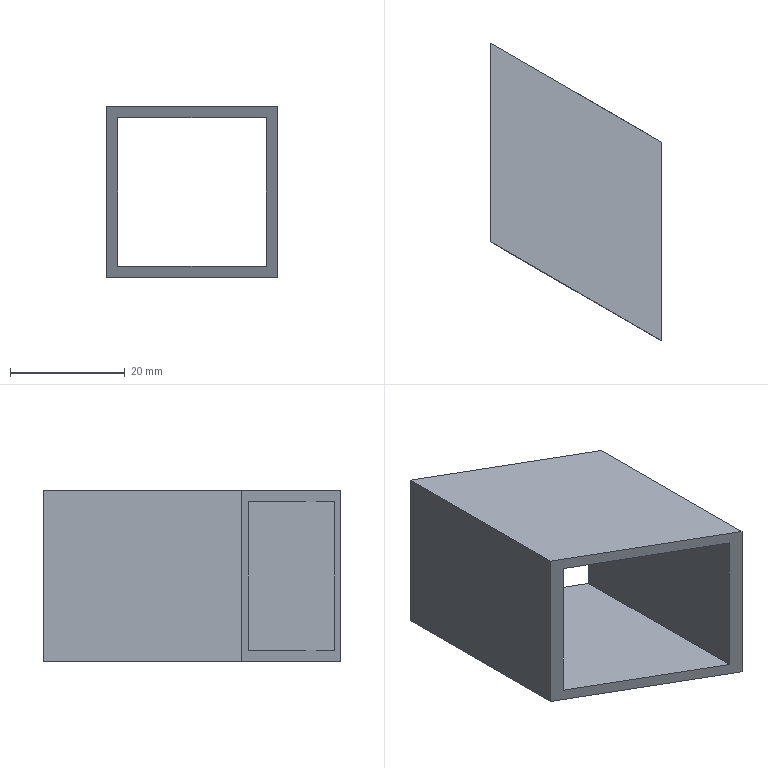Part | NX | features solid 2 | 1 solid | 10 faces | box 30 x 51.962 x 30 mm | volume 7760 mm3 | plane 10
STEP:
#1=CARTESIAN_POINT('',(242.,-18.46,-73.));
#2=VERTEX_POINT('',#1);
#3=CARTESIAN_POINT('',(242.,-18.46,-47.));
#4=VERTEX_POINT('',#3);
#5=CARTESIAN_POINT('',(242.,-18.46,-75.));
#6=DIRECTION('',(0.,0.,1.));
#7=VECTOR('',#6,1000.);
#8=LINE('',#5,#7);
#9=EDGE_CURVE('',#2,#4,#8,.T.);
#10=ORIENTED_EDGE('',*,*,#9,.F.);
#11=CARTESIAN_POINT('',(268.,-33.471,-73.));
#12=VERTEX_POINT('',#11);
#13=CARTESIAN_POINT('',(237.686,-15.97,-73.));
#14=DIRECTION('',(0.866,-0.5,0.));
#15=VECTOR('',#14,1000.);
#16=LINE('',#13,#15);
#17=EDGE_CURVE('',#12,#2,#16,.F.);
#18=ORIENTED_EDGE('',*,*,#17,.F.);
#19=CARTESIAN_POINT('',(268.,-33.471,-47.));
#20=VERTEX_POINT('',#19);
#21=CARTESIAN_POINT('',(268.,-33.471,-75.));
#22=DIRECTION('',(0.,0.,1.));
#23=VECTOR('',#22,1000.);
#24=LINE('',#21,#23);
#25=EDGE_CURVE('',#12,#20,#24,.T.);
#26=ORIENTED_EDGE('',*,*,#25,.T.);
#27=CARTESIAN_POINT('',(237.686,-15.97,-47.));
#28=DIRECTION('',(0.866,-0.5,0.));
#29=VECTOR('',#28,1000.);
#30=LINE('',#27,#29);
#31=EDGE_CURVE('',#4,#20,#30,.T.);
#32=ORIENTED_EDGE('',*,*,#31,.F.);
#33=EDGE_LOOP('',(#10,#18,#26,#32));
#34=FACE_BOUND('',#33,.T.);
#35=CARTESIAN_POINT('',(270.,-34.626,-75.));
#36=VERTEX_POINT('',#35);
#37=CARTESIAN_POINT('',(240.,-17.306,-75.));
#38=VERTEX_POINT('',#37);
#39=CARTESIAN_POINT('',(237.686,-15.97,-75.));
#40=DIRECTION('',(0.866,-0.5,0.));
#41=VECTOR('',#40,1000.);
#42=LINE('',#39,#41);
#43=EDGE_CURVE('',#36,#38,#42,.F.);
#44=ORIENTED_EDGE('',*,*,#43,.T.);
#45=CARTESIAN_POINT('',(240.,-17.306,-45.));
#46=VERTEX_POINT('',#45);
#47=CARTESIAN_POINT('',(240.,-17.306,-75.));
#48=DIRECTION('',(0.,0.,1.));
#49=VECTOR('',#48,1000.);
#50=LINE('',#47,#49);
#51=EDGE_CURVE('',#38,#46,#50,.T.);
#52=ORIENTED_EDGE('',*,*,#51,.T.);
#53=CARTESIAN_POINT('',(270.,-34.626,-45.));
#54=VERTEX_POINT('',#53);
#55=CARTESIAN_POINT('',(237.686,-15.97,-45.));
#56=DIRECTION('',(0.866,-0.5,0.));
#57=VECTOR('',#56,1000.);
#58=LINE('',#55,#57);
#59=EDGE_CURVE('',#46,#54,#58,.T.);
#60=ORIENTED_EDGE('',*,*,#59,.T.);
#61=CARTESIAN_POINT('',(270.,-34.626,-75.));
#62=DIRECTION('',(0.,0.,1.));
#63=VECTOR('',#62,1000.);
#64=LINE('',#61,#63);
#65=EDGE_CURVE('',#36,#54,#64,.T.);
#66=ORIENTED_EDGE('',*,*,#65,.F.);
#67=EDGE_LOOP('',(#44,#52,#60,#66));
#68=FACE_BOUND('',#67,.T.);
#69=CARTESIAN_POINT('',(476.795,-154.019,-105.));
#70=DIRECTION('',(0.5,0.866,0.));
#71=DIRECTION('',(0.,0.,-1.));
#72=AXIS2_PLACEMENT_3D('',#69,#70,#71);
#73=PLANE('',#72);
#74=ADVANCED_FACE('',(#34,#68),#73,.T.);
#75=CARTESIAN_POINT('',(270.,-69.267,-75.));
#76=VERTEX_POINT('',#75);
#77=CARTESIAN_POINT('',(270.,40.,-75.));
#78=DIRECTION('',(0.,1.,0.));
#79=VECTOR('',#78,1000.);
#80=LINE('',#77,#79);
#81=EDGE_CURVE('',#76,#36,#80,.T.);
#82=ORIENTED_EDGE('',*,*,#81,.T.);
#83=ORIENTED_EDGE('',*,*,#65,.T.);
#84=CARTESIAN_POINT('',(270.,-69.267,-45.));
#85=VERTEX_POINT('',#84);
#86=CARTESIAN_POINT('',(270.,40.,-45.));
#87=DIRECTION('',(0.,1.,0.));
#88=VECTOR('',#87,1000.);
#89=LINE('',#86,#88);
#90=EDGE_CURVE('',#85,#54,#89,.T.);
#91=ORIENTED_EDGE('',*,*,#90,.F.);
#92=CARTESIAN_POINT('',(270.,-69.267,-75.));
#93=DIRECTION('',(0.,0.,1.));
#94=VECTOR('',#93,1000.);
#95=LINE('',#92,#94);
#96=EDGE_CURVE('',#76,#85,#95,.T.);
#97=ORIENTED_EDGE('',*,*,#96,.F.);
#98=EDGE_LOOP('',(#82,#83,#91,#97));
#99=FACE_BOUND('',#98,.T.);
#100=CARTESIAN_POINT('',(270.,40.,-75.));
#101=DIRECTION('',(1.,0.,0.));
#102=DIRECTION('',(0.,1.,0.));
#103=AXIS2_PLACEMENT_3D('',#100,#101,#102);
#104=PLANE('',#103);
#105=ADVANCED_FACE('',(#99),#104,.T.);
#106=ORIENTED_EDGE('',*,*,#51,.F.);
#107=CARTESIAN_POINT('',(240.,-51.947,-75.));
#108=VERTEX_POINT('',#107);
#109=CARTESIAN_POINT('',(240.,40.,-75.));
#110=DIRECTION('',(0.,1.,0.));
#111=VECTOR('',#110,1000.);
#112=LINE('',#109,#111);
#113=EDGE_CURVE('',#108,#38,#112,.T.);
#114=ORIENTED_EDGE('',*,*,#113,.F.);
#115=CARTESIAN_POINT('',(240.,-51.947,-45.));
#116=VERTEX_POINT('',#115);
#117=CARTESIAN_POINT('',(240.,-51.947,-75.));
#118=DIRECTION('',(0.,0.,1.));
#119=VECTOR('',#118,1000.);
#120=LINE('',#117,#119);
#121=EDGE_CURVE('',#108,#116,#120,.T.);
#122=ORIENTED_EDGE('',*,*,#121,.T.);
#123=CARTESIAN_POINT('',(240.,40.,-45.));
#124=DIRECTION('',(0.,1.,0.));
#125=VECTOR('',#124,1000.);
#126=LINE('',#123,#125);
#127=EDGE_CURVE('',#116,#46,#126,.T.);
#128=ORIENTED_EDGE('',*,*,#127,.T.);
#129=EDGE_LOOP('',(#106,#114,#122,#128));
#130=FACE_BOUND('',#129,.T.);
#131=CARTESIAN_POINT('',(240.,40.,-75.));
#132=DIRECTION('',(1.,0.,0.));
#133=DIRECTION('',(0.,1.,0.));
#134=AXIS2_PLACEMENT_3D('',#131,#132,#133);
#135=PLANE('',#134);
#136=ADVANCED_FACE('',(#130),#135,.F.);
#137=ORIENTED_EDGE('',*,*,#59,.F.);
#138=ORIENTED_EDGE('',*,*,#127,.F.);
#139=CARTESIAN_POINT('',(461.795,-180.,-45.));
#140=DIRECTION('',(-0.866,0.5,0.));
#141=VECTOR('',#140,1000.);
#142=LINE('',#139,#141);
#143=EDGE_CURVE('',#85,#116,#142,.T.);
#144=ORIENTED_EDGE('',*,*,#143,.F.);
#145=ORIENTED_EDGE('',*,*,#90,.T.);
#146=EDGE_LOOP('',(#137,#138,#144,#145));
#147=FACE_BOUND('',#146,.T.);
#148=CARTESIAN_POINT('',(270.,40.,-45.));
#149=DIRECTION('',(0.,0.,-1.));
#150=DIRECTION('',(0.,1.,0.));
#151=AXIS2_PLACEMENT_3D('',#148,#149,#150);
#152=PLANE('',#151);
#153=ADVANCED_FACE('',(#147),#152,.F.);
#154=ORIENTED_EDGE('',*,*,#43,.F.);
#155=ORIENTED_EDGE('',*,*,#81,.F.);
#156=CARTESIAN_POINT('',(222.686,-41.95,-75.));
#157=DIRECTION('',(0.866,-0.5,0.));
#158=VECTOR('',#157,1000.);
#159=LINE('',#156,#158);
#160=EDGE_CURVE('',#76,#108,#159,.F.);
#161=ORIENTED_EDGE('',*,*,#160,.T.);
#162=ORIENTED_EDGE('',*,*,#113,.T.);
#163=EDGE_LOOP('',(#154,#155,#161,#162));
#164=FACE_BOUND('',#163,.T.);
#165=CARTESIAN_POINT('',(270.,40.,-75.));
#166=DIRECTION('',(0.,0.,-1.));
#167=DIRECTION('',(0.,1.,0.));
#168=AXIS2_PLACEMENT_3D('',#165,#166,#167);
#169=PLANE('',#168);
#170=ADVANCED_FACE('',(#164),#169,.T.);
#171=ORIENTED_EDGE('',*,*,#96,.T.);
#172=ORIENTED_EDGE('',*,*,#143,.T.);
#173=ORIENTED_EDGE('',*,*,#121,.F.);
#174=ORIENTED_EDGE('',*,*,#160,.F.);
#175=EDGE_LOOP('',(#171,#172,#173,#174));
#176=FACE_BOUND('',#175,.T.);
#177=CARTESIAN_POINT('',(268.,-68.112,-73.));
#178=VERTEX_POINT('',#177);
#179=CARTESIAN_POINT('',(268.,-68.112,-47.));
#180=VERTEX_POINT('',#179);
#181=CARTESIAN_POINT('',(268.,-68.112,-75.));
#182=DIRECTION('',(0.,0.,1.));
#183=VECTOR('',#182,1000.);
#184=LINE('',#181,#183);
#185=EDGE_CURVE('',#178,#180,#184,.T.);
#186=ORIENTED_EDGE('',*,*,#185,.F.);
#187=CARTESIAN_POINT('',(242.,-53.101,-73.));
#188=VERTEX_POINT('',#187);
#189=CARTESIAN_POINT('',(222.686,-41.95,-73.));
#190=DIRECTION('',(0.866,-0.5,0.));
#191=VECTOR('',#190,1000.);
#192=LINE('',#189,#191);
#193=EDGE_CURVE('',#178,#188,#192,.F.);
#194=ORIENTED_EDGE('',*,*,#193,.T.);
#195=CARTESIAN_POINT('',(242.,-53.101,-47.));
#196=VERTEX_POINT('',#195);
#197=CARTESIAN_POINT('',(242.,-53.101,-75.));
#198=DIRECTION('',(0.,0.,1.));
#199=VECTOR('',#198,1000.);
#200=LINE('',#197,#199);
#201=EDGE_CURVE('',#188,#196,#200,.T.);
#202=ORIENTED_EDGE('',*,*,#201,.T.);
#203=CARTESIAN_POINT('',(461.795,-180.,-47.));
#204=DIRECTION('',(-0.866,0.5,0.));
#205=VECTOR('',#204,1000.);
#206=LINE('',#203,#205);
#207=EDGE_CURVE('',#180,#196,#206,.T.);
#208=ORIENTED_EDGE('',*,*,#207,.F.);
#209=EDGE_LOOP('',(#186,#194,#202,#208));
#210=FACE_BOUND('',#209,.T.);
#211=CARTESIAN_POINT('',(461.795,-180.,-105.));
#212=DIRECTION('',(0.5,0.866,0.));
#213=DIRECTION('',(0.,0.,-1.));
#214=AXIS2_PLACEMENT_3D('',#211,#212,#213);
#215=PLANE('',#214);
#216=ADVANCED_FACE('',(#176,#210),#215,.F.);
#217=ORIENTED_EDGE('',*,*,#25,.F.);
#218=CARTESIAN_POINT('',(268.,40.,-73.));
#219=DIRECTION('',(0.,-1.,0.));
#220=VECTOR('',#219,1000.);
#221=LINE('',#218,#220);
#222=EDGE_CURVE('',#178,#12,#221,.F.);
#223=ORIENTED_EDGE('',*,*,#222,.F.);
#224=ORIENTED_EDGE('',*,*,#185,.T.);
#225=CARTESIAN_POINT('',(268.,40.,-47.));
#226=DIRECTION('',(0.,1.,0.));
#227=VECTOR('',#226,1000.);
#228=LINE('',#225,#227);
#229=EDGE_CURVE('',#180,#20,#228,.T.);
#230=ORIENTED_EDGE('',*,*,#229,.T.);
#231=EDGE_LOOP('',(#217,#223,#224,#230));
#232=FACE_BOUND('',#231,.T.);
#233=CARTESIAN_POINT('',(268.,40.,-75.));
#234=DIRECTION('',(1.,0.,0.));
#235=DIRECTION('',(0.,1.,0.));
#236=AXIS2_PLACEMENT_3D('',#233,#234,#235);
#237=PLANE('',#236);
#238=ADVANCED_FACE('',(#232),#237,.F.);
#239=CARTESIAN_POINT('',(242.,40.,-73.));
#240=DIRECTION('',(0.,-1.,0.));
#241=VECTOR('',#240,1000.);
#242=LINE('',#239,#241);
#243=EDGE_CURVE('',#188,#2,#242,.F.);
#244=ORIENTED_EDGE('',*,*,#243,.T.);
#245=ORIENTED_EDGE('',*,*,#9,.T.);
#246=CARTESIAN_POINT('',(242.,40.,-47.));
#247=DIRECTION('',(0.,1.,0.));
#248=VECTOR('',#247,1000.);
#249=LINE('',#246,#248);
#250=EDGE_CURVE('',#196,#4,#249,.T.);
#251=ORIENTED_EDGE('',*,*,#250,.F.);
#252=ORIENTED_EDGE('',*,*,#201,.F.);
#253=EDGE_LOOP('',(#244,#245,#251,#252));
#254=FACE_BOUND('',#253,.T.);
#255=CARTESIAN_POINT('',(242.,40.,-75.));
#256=DIRECTION('',(1.,0.,0.));
#257=DIRECTION('',(0.,1.,0.));
#258=AXIS2_PLACEMENT_3D('',#255,#256,#257);
#259=PLANE('',#258);
#260=ADVANCED_FACE('',(#254),#259,.T.);
#261=ORIENTED_EDGE('',*,*,#250,.T.);
#262=ORIENTED_EDGE('',*,*,#31,.T.);
#263=ORIENTED_EDGE('',*,*,#229,.F.);
#264=ORIENTED_EDGE('',*,*,#207,.T.);
#265=EDGE_LOOP('',(#261,#262,#263,#264));
#266=FACE_BOUND('',#265,.T.);
#267=CARTESIAN_POINT('',(270.,40.,-47.));
#268=DIRECTION('',(0.,0.,-1.));
#269=DIRECTION('',(0.,1.,0.));
#270=AXIS2_PLACEMENT_3D('',#267,#268,#269);
#271=PLANE('',#270);
#272=ADVANCED_FACE('',(#266),#271,.T.);
#273=ORIENTED_EDGE('',*,*,#222,.T.);
#274=ORIENTED_EDGE('',*,*,#17,.T.);
#275=ORIENTED_EDGE('',*,*,#243,.F.);
#276=ORIENTED_EDGE('',*,*,#193,.F.);
#277=EDGE_LOOP('',(#273,#274,#275,#276));
#278=FACE_BOUND('',#277,.T.);
#279=CARTESIAN_POINT('',(270.,40.,-73.));
#280=DIRECTION('',(0.,0.,-1.));
#281=DIRECTION('',(0.,1.,0.));
#282=AXIS2_PLACEMENT_3D('',#279,#280,#281);
#283=PLANE('',#282);
#284=ADVANCED_FACE('',(#278),#283,.F.);
#285=CLOSED_SHELL('',(#74,#105,#136,#153,#170,#216,#238,#260,#272,#284));
#286=MANIFOLD_SOLID_BREP('',#285);
#287=(LENGTH_UNIT()NAMED_UNIT(*)SI_UNIT(.MILLI.,.METRE.));
#288=UNCERTAINTY_MEASURE_WITH_UNIT(LENGTH_MEASURE(0.00001),#287,'','');
#289=(NAMED_UNIT(*)PLANE_ANGLE_UNIT()SI_UNIT($,.RADIAN.));
#290=(NAMED_UNIT(*)SI_UNIT($,.STERADIAN.)SOLID_ANGLE_UNIT());
#291=(GEOMETRIC_REPRESENTATION_CONTEXT(3)GLOBAL_UNCERTAINTY_ASSIGNED_CONTEXT((#288))GLOBAL_UNIT_ASSIGNED_CONTEXT((#287,#289,#290))REPRESENTATION_CONTEXT('',''));
#292=ADVANCED_BREP_SHAPE_REPRESENTATION('',(#286),#291);